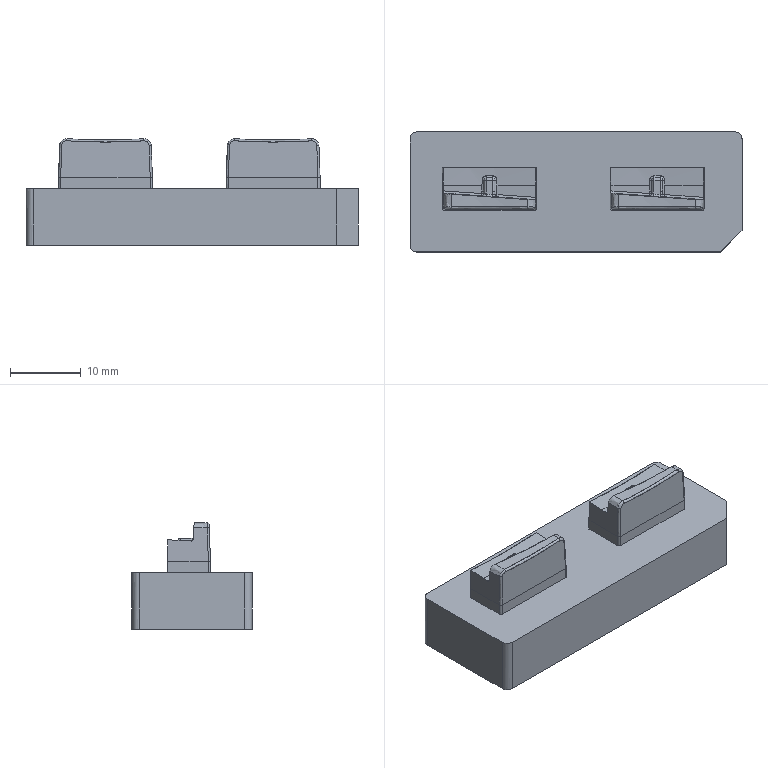NC program | PowerMill | posted with a generic post | part box 47 x 17 x 15.061 mm
Lines 10133 to 10742 of 128250:
N10230 M6
N10231 S8500 M03
N10232 G00 G90 X0.0 Y0.0
N10233 G43 Z9.8009 H3
N10234
N10235 G05 P10000 R8
N10236 X-29.8015 Y-16.545
N10237 Z-6.06
N10238 G01 Z-7.26 F360.0
N10239 X-26.4798 Y-12.4472 F600.0
N10240 X-17.3175 Y-7.866
N10241 X-18.5151
N10242 X-18.909 Y-7.8563
N10243 X-19.303 Y-7.8177
N10244 X-19.6969 Y-7.7548
N10245 X-20.0909 Y-7.6603
N10246 X-20.6541 Y-7.4684
N10247 X-20.8787 Y-7.3724
N10248 X-21.2727 Y-7.177
N10249 X-21.6666 Y-6.9379
N10250 X-22.0198 Y-6.6822
N10251 X-22.4545 Y-6.3037
N10252 X-22.8338 Y-5.8961
N10253 X-23.0521 Y-5.622
N10254 X-23.2424 Y-5.3479
N10255 X-23.3901 Y-5.1099
N10256 X-23.5968 Y-4.7169
N10257 X-23.7679 Y-4.3238
N10258 X-23.904 Y-3.9307
N10259 X-24.0302 Y-3.4317
N10260 X-24.1264 Y-2.7515
N10261 X-24.1449 Y-1.9654
N10262 X-24.1518 Y3.5376
N10263 X-24.1314 Y3.9307
N10264 X-24.0803 Y4.3238
N10265 X-24.0302 Y4.5817
N10266 X-23.8856 Y5.1099
N10267 X-23.7371 Y5.503
N10268 X-23.5509 Y5.8961
N10269 X-23.407 Y6.1533
N10270 X-23.2424 Y6.4104
N10271 X-23.0446 Y6.6822
N10272 X-22.7735 Y7.0024
N10273 X-22.4545 Y7.3225
N10274 X-22.2883 Y7.4684
N10275 X-21.9775 Y7.7114
N10276 X-21.6666 Y7.9198
N10277 X-21.3496 Y8.1012
N10278 X-21.0326 Y8.2545
N10279 X-20.8787 Y8.3198
N10280 X-20.4848 Y8.4619
N10281 X-20.0909 Y8.57
N10282 X-19.6969 Y8.6456
N10283 X-19.303 Y8.6913
N10284 X-18.5151 Y8.7067
N10285 X-5.5151 Y8.7055
N10286 X-5.1212 Y8.6837
N10287 X-4.7273 Y8.6318
N10288 X-4.3333 Y8.5485
N10289 X-3.9394 Y8.4333
N10290 X-3.4793 Y8.2545
N10291 X-3.1184 Y8.0773
N10292 X-2.7576 Y7.8637
N10293 X-2.4906 Y7.6793
N10294 X-2.2236 Y7.4684
N10295 X-1.9697 Y7.2396
N10296 X-1.701 Y6.9609
N10297 X-1.468 Y6.6822
N10298 X-1.1999 Y6.3025
N10299 G03 X0.4365 Y6.3062 I0.8169 J0.5768
N10300 G01 X0.6994 Y6.6822
N10301 X0.9243 Y6.9513
N10302 X1.1818 Y7.2204
N10303 X1.4557 Y7.4684
N10304 X1.7127 Y7.6717
N10305 X1.9697 Y7.8515
N10306 X2.3405 Y8.0721
N10307 X2.7576 Y8.2752
N10308 X3.1515 Y8.4271
N10309 X3.5454 Y8.5439
N10310 X3.9394 Y8.6283
N10311 X4.3333 Y8.6814
N10312 X4.7273 Y8.7049
N10313 X17.7272 Y8.7067
N10314 X18.5151 Y8.6929
N10315 X18.909 Y8.649
N10316 X19.303 Y8.5746
N10317 X19.6969 Y8.4682
N10318 X20.0909 Y8.3282
N10319 X20.2647 Y8.2545
N10320 X20.5717 Y8.1059
N10321 X20.8787 Y7.9321
N10322 X21.1996 Y7.7184
N10323 X21.5204 Y7.4684
N10324 X21.6666 Y7.3402
N10325 X21.9974 Y7.0112
N10326 X22.276 Y6.6822
N10327 X22.4545 Y6.4389
N10328 X22.6302 Y6.1675
N10329 X22.783 Y5.8961
N10330 X22.9688 Y5.503
N10331 X23.117 Y5.1099
N10332 X23.2424 Y4.6677
N10333 X23.3124 Y4.3238
N10334 X23.3629 Y3.9307
N10335 X23.3839 Y3.5376
N10336 X23.377 Y-1.9654
N10337 X23.3586 Y-2.7515
N10338 X23.3132 Y-3.138
N10339 X23.2401 Y-3.5376
N10340 X23.1364 Y-3.9307
N10341 X22.9992 Y-4.3238
N10342 X22.829 Y-4.7169
N10343 X22.6215 Y-5.1099
N10344 X22.4545 Y-5.3786
N10345 X22.2726 Y-5.6374
N10346 X22.0659 Y-5.8961
N10347 X21.8772 Y-6.1091
N10348 X21.6666 Y-6.3222
N10349 X21.2519 Y-6.6822
N10350 X20.8787 Y-6.9509
N10351 X20.4848 Y-7.1877
N10352 X20.0909 Y-7.3808
N10353 X19.8447 Y-7.4844
N10354 X19.5942 Y-7.577
N10355 X19.303 Y-7.6657
N10356 X18.909 Y-7.7584
N10357 X18.5151 Y-7.8207
N10358 X18.1212 Y-7.8578
N10359 X17.7272 Y-7.866
N10360 X5.1212
N10361 X4.7273 Y-7.8491
N10362 X4.3333 Y-7.8039
N10363 X3.9394 Y-7.7318
N10364 X3.5454 Y-7.6288
N10365 X3.09 Y-7.4684
N10366 X2.7576 Y-7.3233
N10367 X2.3636 Y-7.1164
N10368 X1.9697 Y-6.8649
N10369 X1.7243 Y-6.6822
N10370 X1.453 Y-6.4553
N10371 X1.1818 Y-6.1963
N10372 X0.9102 Y-5.8961
N10373 X0.6293 Y-5.5364
N10374 X0.4532 Y-5.2673
N10375 G03 X-1.2174 Y-5.2626 I-0.8368 J-0.5475
N10376 G01 X-1.4093 Y-5.5525
N10377 X-1.6781 Y-5.8961
N10378 X-1.9697 Y-6.2162
N10379 X-2.2309 Y-6.4638
N10380 X-2.4921 Y-6.6822
N10381 X-2.7576 Y-6.878
N10382 X-3.1515 Y-7.1271
N10383 X-3.5454 Y-7.3325
N10384 X-3.8586 Y-7.4684
N10385 X-4.3333 Y-7.635
N10386 X-4.7273 Y-7.7361
N10387 X-5.1212 Y-7.8062
N10388 X-5.5151 Y-7.8506
N10389 X-5.9091 Y-7.866
N10390 X-17.3175
N10391 G00 Z9.8009
N10392 G05 P0
N10393 (---------------)
N10394 ( END TOOLPATH : 粗公基准台01-基准面偏置-D10 )
N10395 (---------------)
N10396 ( START TOOLPATH : 粗公基准台01-外形侧光-D10 )
N10397 (---------------)
N10398 G00 X0.0 Y0.0 Z10.801
N10399 G05 P10000 R8
N10400 X-1.5666 Y-6.0224
N10401 Z-6.03
N10402 G01 Z-7.23 F360.0
N10403 G03 X-2.668 Y-6.3462 I-0.1598 J-1.4915 F600.0
N10404 G02 X-5.808 Y-7.4944 I-3.2567 J4.0386
N10405 G01 X-18.4583 Y-7.4956
N10406 G02 X-23.7743 Y-2.1944 I-0.1254 J5.1903
N10407 G01 X-23.7821 Y3.4877
N10408 G02 X-18.9742 Y8.3355 I4.8799 J-0.0317
N10409 G01 X-12.3913 Y8.3356
N10410 X-5.5471
N10411 G02 X-0.73 Y3.4849 I-0.0629 J-4.8797
N10412 G01 X-0.7378 Y-2.1949
N10413 G02 X-2.668 Y-6.3462 I-5.1869 J-0.1127
N10414 G03 X-3.2179 Y-7.354 I0.9416 J-1.1677
N10415 G01 X-1.6335 Y-5.9798
N10416 G03 X-2.7364 Y-6.2986 I-0.1667 J-1.4907
N10417 G02 X-5.8084 Y-7.4144 I-3.1883 J3.991
N10418 G01 X-18.4579 Y-7.4156
N10419 G02 X-23.6943 Y-2.1943 I-0.1257 J5.1103
N10420 G01 X-23.7021 Y3.4851
N10421 G02 X-18.9742 Y8.2555 I4.7999 J-0.0291
N10422 G01 X-12.3913 Y8.256
N10423 X-5.5503 Y8.2557
N10424 G02 X-0.81 Y3.4851 I-0.0596 J-4.7997
N10425 G01 X-0.8178 Y-2.1943
N10426 G02 X-2.7364 Y-6.2986 I-5.1069 J-0.1133
N10427 G03 X-3.2909 Y-7.3038 I0.9362 J-1.1719
N10428 G00 Z4.0076
N10429 G01 X22.1242 Y-6.0824 F10000.0
N10430 G00 Z-6.03
N10431 G01 Z-7.23 F360.0
N10432 G03 X21.0184 Y-6.3911 I-0.1803 J-1.4891 F600.0
N10433 G02 X17.6834 Y-7.4956 I-3.2038 J4.0865
N10434 G01 X5.2917
N10435 G02 X-0.0304 Y-2.1944 I-0.131 J5.1906
N10436 G01 X-0.0382 Y3.4877
N10437 G02 X0.1407 Y4.7654 I4.8793 J-0.0316
N10438 G02 X0.1504 Y4.8 I4.6956 J-1.3079
N10439 G02 X4.7758 Y8.3356 I4.6914 J-1.3441
N10440 G01 X18.203 Y8.3355
N10441 G02 X23.0139 Y3.4849 I-0.069 J-4.8795
N10442 G01 X23.0061 Y-2.1949
N10443 G02 X21.0184 Y-6.3911 I-5.1915 J-0.1097
N10444 G03 X20.4548 Y-7.3912 I0.9255 J-1.1804
N10445 G01 X22.0579 Y-6.0389
N10446 G03 X20.9507 Y-6.3425 I-0.1871 J-1.4882
N10447 G02 X17.6834 Y-7.4156 I-3.1361 J4.0379
N10448 G01 X5.2921
N10449 G02 X0.0496 Y-2.1943 I-0.1314 J5.1106
N10450 G01 X0.0418 Y3.4851
N10451 G02 X0.2177 Y4.7439 I4.8004 J-0.0291
N10452 G02 X0.2267 Y4.7758 I4.6355 J-1.291
N10453 G02 X4.7758 Y8.2556 I4.615 J-1.3198
N10454 G01 X18.1997
N10455 G02 X22.9339 Y3.4851 I-0.0657 J-4.7995
N10456 G01 X22.9261 Y-2.1943
N10457 G02 X20.9507 Y-6.3425 I-5.1115 J-0.1103
N10458 G03 X20.3825 Y-7.3401 I0.9201 J-1.1846
N10459 G00 Z10.801
N10460 G05 P0
N10461 (---------------)
N10462 ( END TOOLPATH : 粗公基准台01-外形侧光-D10 )
N10463 (---------------)
N10464 ( START TOOLPATH : 粗公基准台01-基准台侧光-D10 )
N10465 (---------------)
N10466 G00 X0.0 Y0.0 Z9.8009
N10467 G05 P10000 R8
N10468 X28.4461 Y-14.8089
N10469 Z-13.96
N10470 G01 Z-15.16 F360.0
N10471 G03 X24.9108 Y-11.2732 I-1.7676 J1.7678 F600.0
N10472 G01 X24.0587 Y-12.1252
N10473 X24.0572 Y-12.1266
N10474 X24.0557 Y-12.128
N10475 X23.7438 Y-12.4094
N10476 X23.7417 Y-12.4112
N10477 X23.7396 Y-12.4129
N10478 X23.5285 Y-12.5785
N10479 X23.5267 Y-12.5799
N10480 X23.5249 Y-12.5812
N10481 X23.2891 Y-12.7459
N10482 X23.2864 Y-12.7477
N10483 X23.2836 Y-12.7493
N10484 X22.8366 Y-13.0106
N10485 X22.8331 Y-13.0126
N10486 X22.8295 Y-13.0144
N10487 X22.3825 Y-13.2182
N10488 X22.3789 Y-13.2197
N10489 X22.3753 Y-13.2211
N10490 X21.9283 Y-13.375
N10491 X21.9247 Y-13.3762
N10492 X21.9211 Y-13.3771
N10493 X21.4655 Y-13.4873
N10494 X21.4619 Y-13.4881
N10495 X21.4583 Y-13.4887
N10496 X21.02 Y-13.5532
N10497 X21.0164 Y-13.5537
N10498 X21.0129 Y-13.554
N10499 X20.5659 Y-13.5795
N10500 X20.5636 Y-13.5796
N10501 X20.5613
N10502 X-22.3493 Y-13.58
N10503 X-22.3501
N10504 X-22.3509
N10505 X-22.7978 Y-13.5712
N10506 X-22.8004
N10507 X-22.803 Y-13.571
N10508 X-23.25 Y-13.5333
N10509 X-23.253 Y-13.5329
N10510 X-23.2561 Y-13.5325
N10511 X-23.7031 Y-13.4598
N10512 X-23.7061 Y-13.4592
N10513 X-23.7092 Y-13.4585
N10514 X-24.1561 Y-13.3498
N10515 X-24.1592 Y-13.349
N10516 X-24.1622 Y-13.3481
N10517 X-24.6091 Y-13.2015
N10518 X-24.6119 Y-13.2005
N10519 X-24.6146 Y-13.1995
N10520 X-25.011 Y-13.0366
N10521 X-25.0142 Y-13.0352
N10522 X-25.0173 Y-13.0337
N10523 X-25.5148 Y-12.7771
N10524 X-25.5172 Y-12.7758
N10525 X-25.5196 Y-12.7745
N10526 X-25.8344 Y-12.584
N10527 X-25.8361 Y-12.583
N10528 X-25.8378 Y-12.5819
N10529 X-25.97 Y-12.4925
N10530 X-25.9721 Y-12.491
N10531 X-25.9743 Y-12.4894
N10532 X-26.4212 Y-12.142
N10533 X-26.4239 Y-12.1398
N10534 X-26.4265 Y-12.1375
N10535 X-26.8735 Y-11.7232
N10536 X-26.8767 Y-11.72
N10537 X-26.8797 Y-11.7168
N10538 X-27.3025 Y-11.2269
N10539 X-27.305 Y-11.2239
N10540 X-27.3073 Y-11.2208
N10541 X-27.6229 Y-10.7738
N10542 X-27.6249 Y-10.7708
N10543 X-27.6268 Y-10.7677
N10544 X-27.8856 Y-10.3208
N10545 X-27.8872 Y-10.3178
N10546 X-27.8887 Y-10.3148
N10547 X-28.0999 Y-9.8679
N10548 X-28.1011 Y-9.8651
N10549 X-28.1022 Y-9.8623
N10550 X-28.2348 Y-9.5166
N10551 X-28.2358 Y-9.5138
N10552 X-28.2368 Y-9.5108
N10553 X-28.4001 Y-8.9626
N10554 X-28.401 Y-8.9594
N10555 X-28.4017 Y-8.9561
N10556 X-28.4954 Y-8.5091
N10557 X-28.496 Y-8.5059
N10558 X-28.4964 Y-8.5027
N10559 X-28.5527 Y-8.0557
N10560 X-28.553 Y-8.053
N10561 X-28.5532 Y-8.0503
N10562 X-28.5789 Y-7.6033
N10563 X-28.579 Y-7.6011
N10564 Y-7.5988
N10565 Y7.5988
N10566 Y7.6011
N10567 X-28.5789 Y7.6033
N10568 X-28.5532 Y8.0503
N10569 X-28.553 Y8.053
N10570 X-28.5527 Y8.0557
N10571 X-28.4964 Y8.5027
N10572 X-28.496 Y8.5059
N10573 X-28.4954 Y8.5091
N10574 X-28.4017 Y8.9561
N10575 X-28.4011 Y8.9589
N10576 X-28.4003 Y8.9617
N10577 X-28.2723 Y9.4087
N10578 X-28.2714 Y9.4118
N10579 X-28.2703 Y9.4148
N10580 X-28.1024 Y9.8618
N10581 X-28.1012 Y9.8649
N10582 X-28.0999 Y9.8679
N10583 X-27.8887 Y10.3148
N10584 X-27.8872 Y10.3178
N10585 X-27.8856 Y10.3208
N10586 X-27.6268 Y10.7677
N10587 X-27.625 Y10.7707
N10588 X-27.6231 Y10.7736
N10589 X-27.3316 Y11.1896
N10590 X-27.3294 Y11.1926
N10591 X-27.3271 Y11.1955
N10592 X-26.9206 Y11.6735
N10593 X-26.9176 Y11.6768
N10594 X-26.9145 Y11.6799
N10595 X-26.439 Y12.1269
N10596 X-26.4363 Y12.1294
N10597 X-26.4334 Y12.1317
N10598 X-25.9743 Y12.4893
N10599 X-25.9722 Y12.4909
N10600 X-25.97 Y12.4925
N10601 X-25.8378 Y12.5819
N10602 X-25.8361 Y12.583
N10603 X-25.8344 Y12.584
N10604 X-25.5196 Y12.7745
N10605 X-25.5174 Y12.7757
N10606 X-25.5152 Y12.7769
N10607 X-25.0683 Y13.0105
N10608 X-25.0651 Y13.0121
N10609 X-25.0619 Y13.0135
N10610 X-24.6149 Y13.1993
N10611 X-24.6121 Y13.2005
N10612 X-24.6091 Y13.2015
N10613 X-24.1622 Y13.3481
N10614 X-24.1592 Y13.349
N10615 X-24.1561 Y13.3498
N10616 X-23.7091 Y13.4585
N10617 X-23.7061 Y13.4592
N10618 X-23.7031 Y13.4597
N10619 X-23.2561 Y13.5325
N10620 X-23.2531 Y13.533
N10621 X-23.25 Y13.5333
N10622 X-22.803 Y13.571
N10623 X-22.8004 Y13.5711
N10624 X-22.7978 Y13.5712
N10625 X-22.3509 Y13.58
N10626 X-22.3501
N10627 X-22.3493
N10628 X0.0
N10629 X22.3493
N10630 X22.3501
N10631 X22.3509
N10632 X22.7978 Y13.5712
N10633 X22.8004 Y13.5711
N10634 X22.803 Y13.5709
N10635 X23.25 Y13.5333
N10636 X23.253 Y13.5329
N10637 X23.2561 Y13.5325
N10638 X23.7031 Y13.4598
N10639 X23.7061 Y13.4592
N10640 X23.7092 Y13.4585
N10641 X24.1561 Y13.3498
N10642 X24.1592 Y13.349
N10643 X24.1622 Y13.3481
N10644 X24.6091 Y13.2015
N10645 X24.6119 Y13.2005
N10646 X24.6146 Y13.1995
N10647 X25.011 Y13.0366
N10648 X25.0142 Y13.0352
N10649 X25.0173 Y13.0337
N10650 X25.5148 Y12.7771
N10651 X25.5172 Y12.7758
N10652 X25.5196 Y12.7745
N10653 X25.8344 Y12.584
N10654 X25.8361 Y12.583
N10655 X25.8378 Y12.5819
N10656 X25.97 Y12.4925
N10657 X25.9721 Y12.491
N10658 X25.9743 Y12.4894
N10659 X26.4212 Y12.142
N10660 X26.4239 Y12.1398
N10661 X26.4265 Y12.1375
N10662 X26.8735 Y11.7232
N10663 X26.8767 Y11.72
N10664 X26.8797 Y11.7168
N10665 X27.3025 Y11.2269
N10666 X27.305 Y11.2239
N10667 X27.3073 Y11.2208
N10668 X27.6229 Y10.7738
N10669 X27.6249 Y10.7708
N10670 X27.6268 Y10.7677
N10671 X27.8856 Y10.3208
N10672 X27.8872 Y10.3178
N10673 X27.8887 Y10.3148
N10674 X28.0999 Y9.8679
N10675 X28.1011 Y9.8651
N10676 X28.1022 Y9.8623
N10677 X28.2348 Y9.5166
N10678 X28.2358 Y9.5138
N10679 X28.2368 Y9.5108
N10680 X28.4001 Y8.9626
N10681 X28.401 Y8.9594
N10682 X28.4017 Y8.9561
N10683 X28.4954 Y8.5091
N10684 X28.496 Y8.5059
N10685 X28.4964 Y8.5027
N10686 X28.5527 Y8.0557
N10687 X28.553 Y8.053
N10688 X28.5532 Y8.0503
N10689 X28.5789 Y7.6033
N10690 X28.579 Y7.6011
N10691 X28.5791 Y7.5988
N10692 X28.58 Y-5.3638
N10693 Y-5.3647
N10694 Y-5.3656
N10695 X28.5704 Y-5.8125
N10696 X28.5702 Y-5.816
N10697 X28.5699 Y-5.8194
N10698 X28.5218 Y-6.2664
N10699 X28.5213 Y-6.27
N10700 X28.5207 Y-6.2735
N10701 X28.4311 Y-6.7205
N10702 X28.4303 Y-6.7241
N10703 X28.4293 Y-6.7277
N10704 X28.296 Y-7.1746
N10705 X28.2952 Y-7.1771
N10706 X28.2944 Y-7.1795
N10707 X28.2351 Y-7.3398
N10708 X28.2344 Y-7.3416
N10709 X28.2337 Y-7.3434
N10710 X28.1119 Y-7.6301
N10711 X28.1105 Y-7.633
N10712 X28.1091 Y-7.636
N10713 X27.8742 Y-8.083
N10714 X27.8729 Y-8.0853
N10715 X27.8715 Y-8.0876
N10716 X27.7813 Y-8.2345
N10717 X27.7801 Y-8.2363
N10718 X27.7789 Y-8.2381
N10719 X27.5713 Y-8.5382
N10720 X27.5695 Y-8.5407
N10721 X27.5677 Y-8.543
N10722 X27.3283 Y-8.8391
N10723 X27.3268 Y-8.8409
N10724 X27.3253 Y-8.8426
N10725 X27.188 Y-8.9935
N10726 X27.1869 Y-8.9948
N10727 X27.1857 Y-8.9961
N10728 X26.8759 Y-9.3083
N10729 X26.8758 Y-9.3084
N10730 X26.8757 Y-9.3085
N10731 X24.9108 Y-11.2732
N10732 G03 X28.4461 Y-14.8089 I1.7677 J-1.7679
N10733 G01 X28.395 Y-14.747
N10734 G03 X24.8596 Y-11.2112 I-1.7677 J1.7679
N10735 G01 X24.0021 Y-12.0686
N10736 X23.6902 Y-12.35
N10737 X23.4791 Y-12.5156
N10738 X23.2433 Y-12.6803
N10739 X22.7963 Y-12.9416
N10740 X22.3493 Y-13.1454
N10741 X21.9023 Y-13.2994
N10742 X21.4467 Y-13.4096
N10743 X21.0083 Y-13.4741
N10744 X20.5613 Y-13.4996
N10745 X-22.3493 Y-13.5
N10746 X-22.7963 Y-13.4913
N10747 X-23.2433 Y-13.4535
N10748 X-23.6902 Y-13.3808
N10749 X-24.1372 Y-13.272
N10750 X-24.5842 Y-13.1255
N10751 X-24.9806 Y-12.9626
N10752 X-25.4782 Y-12.706
N10753 X-25.793 Y-12.5156
N10754 X-25.9252 Y-12.4262
N10755 X-26.3722 Y-12.0789
N10756 X-26.8191 Y-11.6645
N10757 X-27.2419 Y-11.1746
N10758 X-27.5576 Y-10.7277
N10759 X-27.8163 Y-10.2807
N10760 X-28.0275 Y-9.8337
N10761 X-28.1601 Y-9.488
N10762 X-28.3234 Y-8.9397
N10763 X-28.4171 Y-8.4927
N10764 X-28.4734 Y-8.0457
N10765 X-28.499 Y-7.5988
N10766 Y7.5988
N10767 X-28.4734 Y8.0457
N10768 X-28.4171 Y8.4927
N10769 X-28.3234 Y8.9397
N10770 X-28.1954 Y9.3867
N10771 X-28.0275 Y9.8337
N10772 X-27.8163 Y10.2807
N10773 X-27.5576 Y10.7277
N10774 X-27.2661 Y11.1437
N10775 X-26.8597 Y11.6216
N10776 X-26.3842 Y12.0686
N10777 X-25.9252 Y12.4262
N10778 X-25.793 Y12.5156
N10779 X-25.4782 Y12.706
N10780 X-25.0312 Y12.9396
N10781 X-24.5842 Y13.1255
N10782 X-24.1372 Y13.272
N10783 X-23.6902 Y13.3808
N10784 X-23.2433 Y13.4536
N10785 X-22.7963 Y13.4912
N10786 X-22.3493 Y13.5
N10787 X0.0
N10788 X22.3493
N10789 X22.7963 Y13.4912
N10790 X23.2433 Y13.4535
N10791 X23.6902 Y13.3808
N10792 X24.1372 Y13.272
N10793 X24.5842 Y13.1255
N10794 X24.9806 Y12.9626
N10795 X25.4782 Y12.706
N10796 X25.793 Y12.5156
N10797 X25.9252 Y12.4262
N10798 X26.3722 Y12.0789
N10799 X26.8191 Y11.6645
N10800 X27.2419 Y11.1746
N10801 X27.5576 Y10.7277
N10802 X27.8163 Y10.2807
N10803 X28.0275 Y9.8337
N10804 X28.1601 Y9.488
N10805 X28.3234 Y8.9397
N10806 X28.4171 Y8.4927
N10807 X28.4734 Y8.0457
N10808 X28.4991 Y7.5988
N10809 X28.5 Y-5.3638
N10810 X28.4904 Y-5.8108
N10811 X28.4422 Y-6.2578
N10812 X28.3527 Y-6.7048
N10813 X28.2193 Y-7.1518
N10814 X28.1601 Y-7.3121
N10815 X28.0382 Y-7.5988
N10816 X27.8034 Y-8.0457
N10817 X27.7131 Y-8.1926
N10818 X27.5055 Y-8.4927
N10819 X27.2661 Y-8.7888
N10820 X27.1289 Y-8.9397
N10821 X26.8191 Y-9.252
N10822 X24.8596 Y-11.2112
N10823 G03 X28.395 Y-14.747 I1.7677 J-1.7679
N10824 G00 Z9.8009
N10825 G05 P0
N10826 (---------------)
N10827 ( END TOOLPATH : 粗公基准台01-基准台侧光-D10 )
N10828 (---------------)
N10829
N10830 M05
N10831 G53 Z0.0
N10832 (---------------)
N10833 ( START TOOLPATH : 粗公精光01-浅滩和陡峭-R1 )
N10834 (---------------)
N10835 ( TOOL NO.    :4 )
N10836 ( TOOL TYPE   : BALLNOSED)
N10837 ( TOOL ID     : R1_2_1)
N10838 ( TOOL DIA    : 2.0 LENGTH 61.68)
N10839 T4